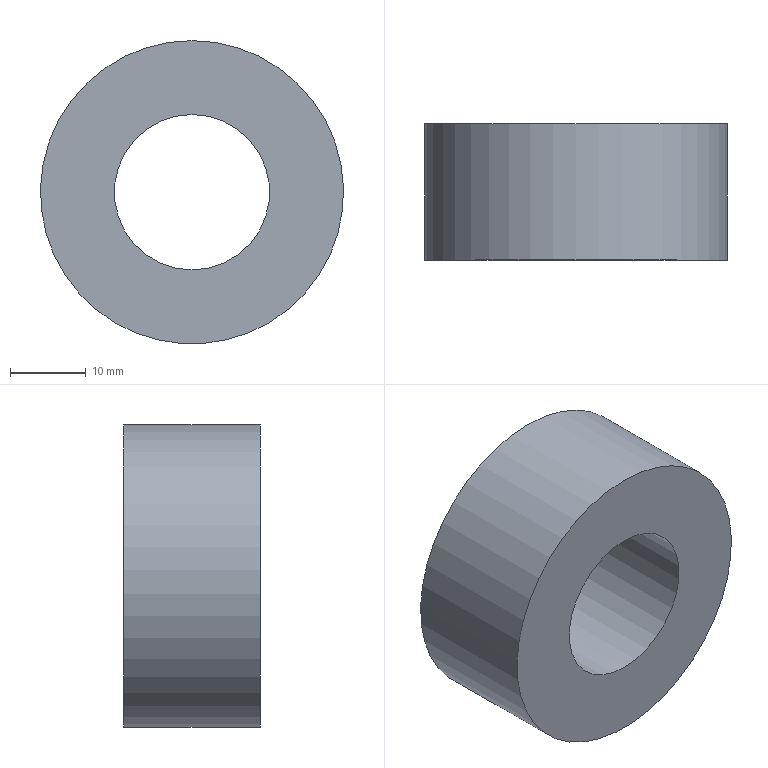Part | NX | 1 solid | 4 faces | box 40 x 18 x 40 mm | volume 16678 mm3 | plane 2 | cylinder 2 | commonest cylinder face diameters 20.5 x1 40 x1
STEP:
#1=CARTESIAN_POINT('',(0.,18.,20.));
#2=VERTEX_POINT('',#1);
#3=CARTESIAN_POINT('',(0.,18.,0.));
#4=DIRECTION('',(0.,1.,0.));
#5=DIRECTION('',(0.,0.,1.));
#6=AXIS2_PLACEMENT_3D('',#3,#4,#5);
#7=CIRCLE('',#6,20.);
#8=EDGE_CURVE('',#2,#2,#7,.T.);
#9=ORIENTED_EDGE('',*,*,#8,.T.);
#10=EDGE_LOOP('',(#9));
#11=FACE_BOUND('',#10,.T.);
#12=CARTESIAN_POINT('',(0.,18.,10.25));
#13=VERTEX_POINT('',#12);
#14=CARTESIAN_POINT('',(0.,18.,0.));
#15=DIRECTION('',(0.,1.,0.));
#16=DIRECTION('',(0.,0.,1.));
#17=AXIS2_PLACEMENT_3D('',#14,#15,#16);
#18=CIRCLE('',#17,10.25);
#19=EDGE_CURVE('',#13,#13,#18,.T.);
#20=ORIENTED_EDGE('',*,*,#19,.F.);
#21=EDGE_LOOP('',(#20));
#22=FACE_BOUND('',#21,.T.);
#23=CARTESIAN_POINT('',(0.,18.,0.));
#24=DIRECTION('',(0.,1.,0.));
#25=DIRECTION('',(0.,0.,1.));
#26=AXIS2_PLACEMENT_3D('',#23,#24,#25);
#27=PLANE('',#26);
#28=ADVANCED_FACE('',(#11,#22),#27,.T.);
#29=CARTESIAN_POINT('',(0.,0.,20.));
#30=VERTEX_POINT('',#29);
#31=CARTESIAN_POINT('',(0.,0.,0.));
#32=DIRECTION('',(0.,1.,0.));
#33=DIRECTION('',(0.,0.,1.));
#34=AXIS2_PLACEMENT_3D('',#31,#32,#33);
#35=CIRCLE('',#34,20.);
#36=EDGE_CURVE('',#30,#30,#35,.T.);
#37=ORIENTED_EDGE('',*,*,#36,.F.);
#38=EDGE_LOOP('',(#37));
#39=FACE_BOUND('',#38,.T.);
#40=CARTESIAN_POINT('',(0.,0.,10.25));
#41=VERTEX_POINT('',#40);
#42=CARTESIAN_POINT('',(0.,0.,0.));
#43=DIRECTION('',(0.,1.,0.));
#44=DIRECTION('',(0.,0.,1.));
#45=AXIS2_PLACEMENT_3D('',#42,#43,#44);
#46=CIRCLE('',#45,10.25);
#47=EDGE_CURVE('',#41,#41,#46,.T.);
#48=ORIENTED_EDGE('',*,*,#47,.T.);
#49=EDGE_LOOP('',(#48));
#50=FACE_BOUND('',#49,.T.);
#51=CARTESIAN_POINT('',(0.,0.,0.));
#52=DIRECTION('',(0.,1.,0.));
#53=DIRECTION('',(0.,0.,1.));
#54=AXIS2_PLACEMENT_3D('',#51,#52,#53);
#55=PLANE('',#54);
#56=ADVANCED_FACE('',(#39,#50),#55,.F.);
#57=ORIENTED_EDGE('',*,*,#8,.F.);
#58=EDGE_LOOP('',(#57));
#59=FACE_BOUND('',#58,.T.);
#60=ORIENTED_EDGE('',*,*,#36,.T.);
#61=EDGE_LOOP('',(#60));
#62=FACE_BOUND('',#61,.T.);
#63=CARTESIAN_POINT('',(0.,18.,0.));
#64=DIRECTION('',(0.,-1.,0.));
#65=DIRECTION('',(0.,0.,-1.));
#66=AXIS2_PLACEMENT_3D('',#63,#64,#65);
#67=CYLINDRICAL_SURFACE('',#66,20.);
#68=ADVANCED_FACE('',(#59,#62),#67,.T.);
#69=ORIENTED_EDGE('',*,*,#19,.T.);
#70=EDGE_LOOP('',(#69));
#71=FACE_BOUND('',#70,.T.);
#72=ORIENTED_EDGE('',*,*,#47,.F.);
#73=EDGE_LOOP('',(#72));
#74=FACE_BOUND('',#73,.T.);
#75=CARTESIAN_POINT('',(0.,18.,0.));
#76=DIRECTION('',(0.,-1.,0.));
#77=DIRECTION('',(0.,0.,-1.));
#78=AXIS2_PLACEMENT_3D('',#75,#76,#77);
#79=CYLINDRICAL_SURFACE('',#78,10.25);
#80=ADVANCED_FACE('',(#71,#74),#79,.F.);
#81=CLOSED_SHELL('',(#28,#56,#68,#80));
#82=MANIFOLD_SOLID_BREP('',#81);
#83=(LENGTH_UNIT()NAMED_UNIT(*)SI_UNIT(.MILLI.,.METRE.));
#84=UNCERTAINTY_MEASURE_WITH_UNIT(LENGTH_MEASURE(0.00001),#83,'','');
#85=(NAMED_UNIT(*)PLANE_ANGLE_UNIT()SI_UNIT($,.RADIAN.));
#86=(NAMED_UNIT(*)SI_UNIT($,.STERADIAN.)SOLID_ANGLE_UNIT());
#87=(GEOMETRIC_REPRESENTATION_CONTEXT(3)GLOBAL_UNCERTAINTY_ASSIGNED_CONTEXT((#84))GLOBAL_UNIT_ASSIGNED_CONTEXT((#83,#85,#86))REPRESENTATION_CONTEXT('',''));
#88=ADVANCED_BREP_SHAPE_REPRESENTATION('',(#82),#87);